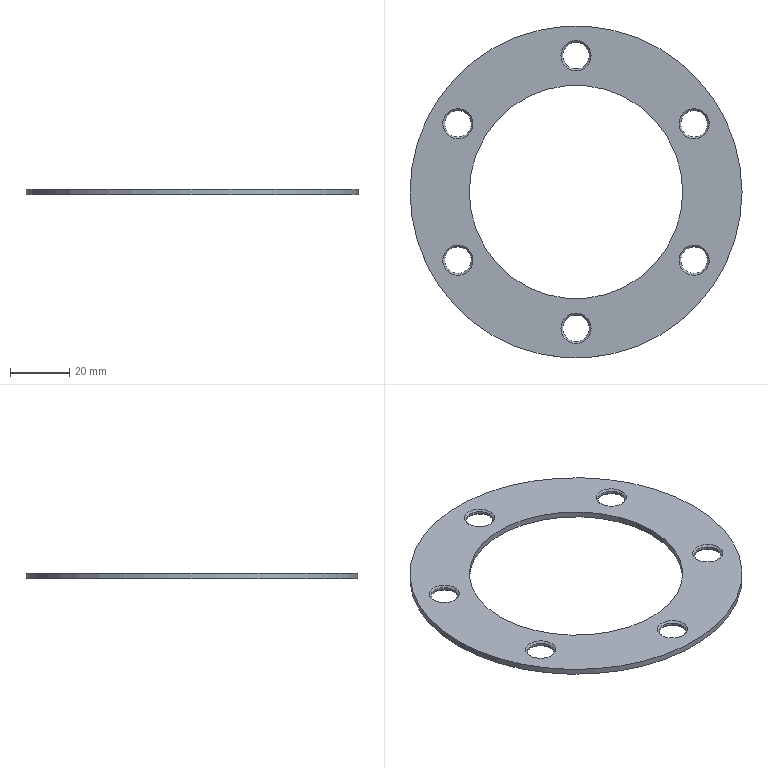Part | NX | 1 solid | 22 faces | box 112 x 112 x 2 mm | volume 10734 mm3 | cone 12 | cylinder 8 | plane 2 | commonest cylinder face diameters 9 x6 72 x1 112 x1
STEP:
#1=CARTESIAN_POINT('',(-37.287,27.417,2.));
#2=VERTEX_POINT('',#1);
#3=CARTESIAN_POINT('',(-39.837,23.,2.));
#4=DIRECTION('',(0.,0.,-1.));
#5=DIRECTION('',(0.5,0.866,0.));
#6=AXIS2_PLACEMENT_3D('',#3,#4,#5);
#7=CIRCLE('',#6,5.1);
#8=EDGE_CURVE('',#2,#2,#7,.T.);
#9=ORIENTED_EDGE('',*,*,#8,.F.);
#10=EDGE_LOOP('',(#9));
#11=FACE_BOUND('',#10,.T.);
#12=CARTESIAN_POINT('',(-37.587,26.897,1.4));
#13=VERTEX_POINT('',#12);
#14=CARTESIAN_POINT('',(-39.837,23.,1.4));
#15=DIRECTION('',(0.,0.,1.));
#16=DIRECTION('',(0.5,0.866,0.));
#17=AXIS2_PLACEMENT_3D('',#14,#15,#16);
#18=CIRCLE('',#17,4.5);
#19=EDGE_CURVE('',#13,#13,#18,.T.);
#20=ORIENTED_EDGE('',*,*,#19,.F.);
#21=EDGE_LOOP('',(#20));
#22=FACE_BOUND('',#21,.T.);
#23=CARTESIAN_POINT('',(-39.837,23.,1.4));
#24=DIRECTION('',(0.,0.,1.));
#25=DIRECTION('',(-0.5,-0.866,0.));
#26=AXIS2_PLACEMENT_3D('',#23,#24,#25);
#27=CONICAL_SURFACE('',#26,4.5,45.);
#28=ADVANCED_FACE('',(#11,#22),#27,.F.);
#29=CARTESIAN_POINT('',(-37.587,26.897,0.6));
#30=VERTEX_POINT('',#29);
#31=CARTESIAN_POINT('',(-39.837,23.,0.6));
#32=DIRECTION('',(0.,0.,-1.));
#33=DIRECTION('',(0.5,0.866,0.));
#34=AXIS2_PLACEMENT_3D('',#31,#32,#33);
#35=CIRCLE('',#34,4.5);
#36=EDGE_CURVE('',#30,#30,#35,.T.);
#37=ORIENTED_EDGE('',*,*,#36,.F.);
#38=EDGE_LOOP('',(#37));
#39=FACE_BOUND('',#38,.T.);
#40=CARTESIAN_POINT('',(-37.287,27.417,0.));
#41=VERTEX_POINT('',#40);
#42=CARTESIAN_POINT('',(-39.837,23.,0.));
#43=DIRECTION('',(0.,0.,1.));
#44=DIRECTION('',(0.5,0.866,0.));
#45=AXIS2_PLACEMENT_3D('',#42,#43,#44);
#46=CIRCLE('',#45,5.1);
#47=EDGE_CURVE('',#41,#41,#46,.T.);
#48=ORIENTED_EDGE('',*,*,#47,.F.);
#49=EDGE_LOOP('',(#48));
#50=FACE_BOUND('',#49,.T.);
#51=CARTESIAN_POINT('',(-39.837,23.,0.));
#52=DIRECTION('',(0.,0.,-1.));
#53=DIRECTION('',(0.5,0.866,0.));
#54=AXIS2_PLACEMENT_3D('',#51,#52,#53);
#55=CONICAL_SURFACE('',#54,5.1,45.);
#56=ADVANCED_FACE('',(#39,#50),#55,.F.);
#57=ORIENTED_EDGE('',*,*,#19,.T.);
#58=EDGE_LOOP('',(#57));
#59=FACE_BOUND('',#58,.T.);
#60=ORIENTED_EDGE('',*,*,#36,.T.);
#61=EDGE_LOOP('',(#60));
#62=FACE_BOUND('',#61,.T.);
#63=CARTESIAN_POINT('',(-39.837,23.,0.));
#64=DIRECTION('',(0.,0.,1.));
#65=DIRECTION('',(-0.5,-0.866,0.));
#66=AXIS2_PLACEMENT_3D('',#63,#64,#65);
#67=CYLINDRICAL_SURFACE('',#66,4.5);
#68=ADVANCED_FACE('',(#59,#62),#67,.F.);
#69=CARTESIAN_POINT('',(-42.387,-18.583,2.));
#70=VERTEX_POINT('',#69);
#71=CARTESIAN_POINT('',(-39.837,-23.,2.));
#72=DIRECTION('',(0.,0.,-1.));
#73=DIRECTION('',(-0.5,0.866,0.));
#74=AXIS2_PLACEMENT_3D('',#71,#72,#73);
#75=CIRCLE('',#74,5.1);
#76=EDGE_CURVE('',#70,#70,#75,.T.);
#77=ORIENTED_EDGE('',*,*,#76,.F.);
#78=EDGE_LOOP('',(#77));
#79=FACE_BOUND('',#78,.T.);
#80=CARTESIAN_POINT('',(-42.087,-19.103,1.4));
#81=VERTEX_POINT('',#80);
#82=CARTESIAN_POINT('',(-39.837,-23.,1.4));
#83=DIRECTION('',(0.,0.,1.));
#84=DIRECTION('',(-0.5,0.866,0.));
#85=AXIS2_PLACEMENT_3D('',#82,#83,#84);
#86=CIRCLE('',#85,4.5);
#87=EDGE_CURVE('',#81,#81,#86,.T.);
#88=ORIENTED_EDGE('',*,*,#87,.F.);
#89=EDGE_LOOP('',(#88));
#90=FACE_BOUND('',#89,.T.);
#91=CARTESIAN_POINT('',(-39.837,-23.,1.4));
#92=DIRECTION('',(0.,0.,1.));
#93=DIRECTION('',(0.5,-0.866,0.));
#94=AXIS2_PLACEMENT_3D('',#91,#92,#93);
#95=CONICAL_SURFACE('',#94,4.5,45.);
#96=ADVANCED_FACE('',(#79,#90),#95,.F.);
#97=CARTESIAN_POINT('',(-42.087,-19.103,0.6));
#98=VERTEX_POINT('',#97);
#99=CARTESIAN_POINT('',(-39.837,-23.,0.6));
#100=DIRECTION('',(0.,0.,-1.));
#101=DIRECTION('',(-0.5,0.866,0.));
#102=AXIS2_PLACEMENT_3D('',#99,#100,#101);
#103=CIRCLE('',#102,4.5);
#104=EDGE_CURVE('',#98,#98,#103,.T.);
#105=ORIENTED_EDGE('',*,*,#104,.F.);
#106=EDGE_LOOP('',(#105));
#107=FACE_BOUND('',#106,.T.);
#108=CARTESIAN_POINT('',(-42.387,-18.583,0.));
#109=VERTEX_POINT('',#108);
#110=CARTESIAN_POINT('',(-39.837,-23.,0.));
#111=DIRECTION('',(0.,0.,1.));
#112=DIRECTION('',(-0.5,0.866,0.));
#113=AXIS2_PLACEMENT_3D('',#110,#111,#112);
#114=CIRCLE('',#113,5.1);
#115=EDGE_CURVE('',#109,#109,#114,.T.);
#116=ORIENTED_EDGE('',*,*,#115,.F.);
#117=EDGE_LOOP('',(#116));
#118=FACE_BOUND('',#117,.T.);
#119=CARTESIAN_POINT('',(-39.837,-23.,0.));
#120=DIRECTION('',(0.,0.,-1.));
#121=DIRECTION('',(-0.5,0.866,0.));
#122=AXIS2_PLACEMENT_3D('',#119,#120,#121);
#123=CONICAL_SURFACE('',#122,5.1,45.);
#124=ADVANCED_FACE('',(#107,#118),#123,.F.);
#125=ORIENTED_EDGE('',*,*,#87,.T.);
#126=EDGE_LOOP('',(#125));
#127=FACE_BOUND('',#126,.T.);
#128=ORIENTED_EDGE('',*,*,#104,.T.);
#129=EDGE_LOOP('',(#128));
#130=FACE_BOUND('',#129,.T.);
#131=CARTESIAN_POINT('',(-39.837,-23.,0.));
#132=DIRECTION('',(0.,0.,1.));
#133=DIRECTION('',(0.5,-0.866,0.));
#134=AXIS2_PLACEMENT_3D('',#131,#132,#133);
#135=CYLINDRICAL_SURFACE('',#134,4.5);
#136=ADVANCED_FACE('',(#127,#130),#135,.F.);
#137=CARTESIAN_POINT('',(-5.1,-46.,2.));
#138=VERTEX_POINT('',#137);
#139=CARTESIAN_POINT('',(0.,-46.,2.));
#140=DIRECTION('',(0.,0.,-1.));
#141=DIRECTION('',(-1.,0.,0.));
#142=AXIS2_PLACEMENT_3D('',#139,#140,#141);
#143=CIRCLE('',#142,5.1);
#144=EDGE_CURVE('',#138,#138,#143,.T.);
#145=ORIENTED_EDGE('',*,*,#144,.F.);
#146=EDGE_LOOP('',(#145));
#147=FACE_BOUND('',#146,.T.);
#148=CARTESIAN_POINT('',(-4.5,-46.,1.4));
#149=VERTEX_POINT('',#148);
#150=CARTESIAN_POINT('',(0.,-46.,1.4));
#151=DIRECTION('',(0.,0.,1.));
#152=DIRECTION('',(-1.,0.,0.));
#153=AXIS2_PLACEMENT_3D('',#150,#151,#152);
#154=CIRCLE('',#153,4.5);
#155=EDGE_CURVE('',#149,#149,#154,.T.);
#156=ORIENTED_EDGE('',*,*,#155,.F.);
#157=EDGE_LOOP('',(#156));
#158=FACE_BOUND('',#157,.T.);
#159=CARTESIAN_POINT('',(0.,-46.,1.4));
#160=DIRECTION('',(0.,0.,1.));
#161=DIRECTION('',(1.,0.,0.));
#162=AXIS2_PLACEMENT_3D('',#159,#160,#161);
#163=CONICAL_SURFACE('',#162,4.5,45.);
#164=ADVANCED_FACE('',(#147,#158),#163,.F.);
#165=CARTESIAN_POINT('',(-4.5,-46.,0.6));
#166=VERTEX_POINT('',#165);
#167=CARTESIAN_POINT('',(0.,-46.,0.6));
#168=DIRECTION('',(0.,0.,-1.));
#169=DIRECTION('',(-1.,0.,0.));
#170=AXIS2_PLACEMENT_3D('',#167,#168,#169);
#171=CIRCLE('',#170,4.5);
#172=EDGE_CURVE('',#166,#166,#171,.T.);
#173=ORIENTED_EDGE('',*,*,#172,.F.);
#174=EDGE_LOOP('',(#173));
#175=FACE_BOUND('',#174,.T.);
#176=CARTESIAN_POINT('',(-5.1,-46.,0.));
#177=VERTEX_POINT('',#176);
#178=CARTESIAN_POINT('',(0.,-46.,0.));
#179=DIRECTION('',(0.,0.,1.));
#180=DIRECTION('',(-1.,0.,0.));
#181=AXIS2_PLACEMENT_3D('',#178,#179,#180);
#182=CIRCLE('',#181,5.1);
#183=EDGE_CURVE('',#177,#177,#182,.T.);
#184=ORIENTED_EDGE('',*,*,#183,.F.);
#185=EDGE_LOOP('',(#184));
#186=FACE_BOUND('',#185,.T.);
#187=CARTESIAN_POINT('',(0.,-46.,0.));
#188=DIRECTION('',(0.,0.,-1.));
#189=DIRECTION('',(-1.,0.,0.));
#190=AXIS2_PLACEMENT_3D('',#187,#188,#189);
#191=CONICAL_SURFACE('',#190,5.1,45.);
#192=ADVANCED_FACE('',(#175,#186),#191,.F.);
#193=ORIENTED_EDGE('',*,*,#155,.T.);
#194=EDGE_LOOP('',(#193));
#195=FACE_BOUND('',#194,.T.);
#196=ORIENTED_EDGE('',*,*,#172,.T.);
#197=EDGE_LOOP('',(#196));
#198=FACE_BOUND('',#197,.T.);
#199=CARTESIAN_POINT('',(0.,-46.,0.));
#200=DIRECTION('',(0.,0.,1.));
#201=DIRECTION('',(1.,0.,0.));
#202=AXIS2_PLACEMENT_3D('',#199,#200,#201);
#203=CYLINDRICAL_SURFACE('',#202,4.5);
#204=ADVANCED_FACE('',(#195,#198),#203,.F.);
#205=CARTESIAN_POINT('',(37.287,-27.417,2.));
#206=VERTEX_POINT('',#205);
#207=CARTESIAN_POINT('',(39.837,-23.,2.));
#208=DIRECTION('',(0.,0.,-1.));
#209=DIRECTION('',(-0.5,-0.866,0.));
#210=AXIS2_PLACEMENT_3D('',#207,#208,#209);
#211=CIRCLE('',#210,5.1);
#212=EDGE_CURVE('',#206,#206,#211,.T.);
#213=ORIENTED_EDGE('',*,*,#212,.F.);
#214=EDGE_LOOP('',(#213));
#215=FACE_BOUND('',#214,.T.);
#216=CARTESIAN_POINT('',(37.587,-26.897,1.4));
#217=VERTEX_POINT('',#216);
#218=CARTESIAN_POINT('',(39.837,-23.,1.4));
#219=DIRECTION('',(0.,0.,1.));
#220=DIRECTION('',(-0.5,-0.866,0.));
#221=AXIS2_PLACEMENT_3D('',#218,#219,#220);
#222=CIRCLE('',#221,4.5);
#223=EDGE_CURVE('',#217,#217,#222,.T.);
#224=ORIENTED_EDGE('',*,*,#223,.F.);
#225=EDGE_LOOP('',(#224));
#226=FACE_BOUND('',#225,.T.);
#227=CARTESIAN_POINT('',(39.837,-23.,1.4));
#228=DIRECTION('',(0.,0.,1.));
#229=DIRECTION('',(0.5,0.866,0.));
#230=AXIS2_PLACEMENT_3D('',#227,#228,#229);
#231=CONICAL_SURFACE('',#230,4.5,45.);
#232=ADVANCED_FACE('',(#215,#226),#231,.F.);
#233=CARTESIAN_POINT('',(37.587,-26.897,0.6));
#234=VERTEX_POINT('',#233);
#235=CARTESIAN_POINT('',(39.837,-23.,0.6));
#236=DIRECTION('',(0.,0.,-1.));
#237=DIRECTION('',(-0.5,-0.866,0.));
#238=AXIS2_PLACEMENT_3D('',#235,#236,#237);
#239=CIRCLE('',#238,4.5);
#240=EDGE_CURVE('',#234,#234,#239,.T.);
#241=ORIENTED_EDGE('',*,*,#240,.F.);
#242=EDGE_LOOP('',(#241));
#243=FACE_BOUND('',#242,.T.);
#244=CARTESIAN_POINT('',(37.287,-27.417,0.));
#245=VERTEX_POINT('',#244);
#246=CARTESIAN_POINT('',(39.837,-23.,0.));
#247=DIRECTION('',(0.,0.,1.));
#248=DIRECTION('',(-0.5,-0.866,0.));
#249=AXIS2_PLACEMENT_3D('',#246,#247,#248);
#250=CIRCLE('',#249,5.1);
#251=EDGE_CURVE('',#245,#245,#250,.T.);
#252=ORIENTED_EDGE('',*,*,#251,.F.);
#253=EDGE_LOOP('',(#252));
#254=FACE_BOUND('',#253,.T.);
#255=CARTESIAN_POINT('',(39.837,-23.,0.));
#256=DIRECTION('',(0.,0.,-1.));
#257=DIRECTION('',(-0.5,-0.866,0.));
#258=AXIS2_PLACEMENT_3D('',#255,#256,#257);
#259=CONICAL_SURFACE('',#258,5.1,45.);
#260=ADVANCED_FACE('',(#243,#254),#259,.F.);
#261=ORIENTED_EDGE('',*,*,#223,.T.);
#262=EDGE_LOOP('',(#261));
#263=FACE_BOUND('',#262,.T.);
#264=ORIENTED_EDGE('',*,*,#240,.T.);
#265=EDGE_LOOP('',(#264));
#266=FACE_BOUND('',#265,.T.);
#267=CARTESIAN_POINT('',(39.837,-23.,0.));
#268=DIRECTION('',(0.,0.,1.));
#269=DIRECTION('',(0.5,0.866,0.));
#270=AXIS2_PLACEMENT_3D('',#267,#268,#269);
#271=CYLINDRICAL_SURFACE('',#270,4.5);
#272=ADVANCED_FACE('',(#263,#266),#271,.F.);
#273=CARTESIAN_POINT('',(42.387,18.583,2.));
#274=VERTEX_POINT('',#273);
#275=CARTESIAN_POINT('',(39.837,23.,2.));
#276=DIRECTION('',(0.,0.,-1.));
#277=DIRECTION('',(0.5,-0.866,0.));
#278=AXIS2_PLACEMENT_3D('',#275,#276,#277);
#279=CIRCLE('',#278,5.1);
#280=EDGE_CURVE('',#274,#274,#279,.T.);
#281=ORIENTED_EDGE('',*,*,#280,.F.);
#282=EDGE_LOOP('',(#281));
#283=FACE_BOUND('',#282,.T.);
#284=CARTESIAN_POINT('',(42.087,19.103,1.4));
#285=VERTEX_POINT('',#284);
#286=CARTESIAN_POINT('',(39.837,23.,1.4));
#287=DIRECTION('',(0.,0.,1.));
#288=DIRECTION('',(0.5,-0.866,0.));
#289=AXIS2_PLACEMENT_3D('',#286,#287,#288);
#290=CIRCLE('',#289,4.5);
#291=EDGE_CURVE('',#285,#285,#290,.T.);
#292=ORIENTED_EDGE('',*,*,#291,.F.);
#293=EDGE_LOOP('',(#292));
#294=FACE_BOUND('',#293,.T.);
#295=CARTESIAN_POINT('',(39.837,23.,1.4));
#296=DIRECTION('',(0.,0.,1.));
#297=DIRECTION('',(-0.5,0.866,0.));
#298=AXIS2_PLACEMENT_3D('',#295,#296,#297);
#299=CONICAL_SURFACE('',#298,4.5,45.);
#300=ADVANCED_FACE('',(#283,#294),#299,.F.);
#301=CARTESIAN_POINT('',(42.087,19.103,0.6));
#302=VERTEX_POINT('',#301);
#303=CARTESIAN_POINT('',(39.837,23.,0.6));
#304=DIRECTION('',(0.,0.,-1.));
#305=DIRECTION('',(0.5,-0.866,0.));
#306=AXIS2_PLACEMENT_3D('',#303,#304,#305);
#307=CIRCLE('',#306,4.5);
#308=EDGE_CURVE('',#302,#302,#307,.T.);
#309=ORIENTED_EDGE('',*,*,#308,.F.);
#310=EDGE_LOOP('',(#309));
#311=FACE_BOUND('',#310,.T.);
#312=CARTESIAN_POINT('',(42.387,18.583,0.));
#313=VERTEX_POINT('',#312);
#314=CARTESIAN_POINT('',(39.837,23.,0.));
#315=DIRECTION('',(0.,0.,1.));
#316=DIRECTION('',(0.5,-0.866,0.));
#317=AXIS2_PLACEMENT_3D('',#314,#315,#316);
#318=CIRCLE('',#317,5.1);
#319=EDGE_CURVE('',#313,#313,#318,.T.);
#320=ORIENTED_EDGE('',*,*,#319,.F.);
#321=EDGE_LOOP('',(#320));
#322=FACE_BOUND('',#321,.T.);
#323=CARTESIAN_POINT('',(39.837,23.,0.));
#324=DIRECTION('',(0.,0.,-1.));
#325=DIRECTION('',(0.5,-0.866,0.));
#326=AXIS2_PLACEMENT_3D('',#323,#324,#325);
#327=CONICAL_SURFACE('',#326,5.1,45.);
#328=ADVANCED_FACE('',(#311,#322),#327,.F.);
#329=ORIENTED_EDGE('',*,*,#291,.T.);
#330=EDGE_LOOP('',(#329));
#331=FACE_BOUND('',#330,.T.);
#332=ORIENTED_EDGE('',*,*,#308,.T.);
#333=EDGE_LOOP('',(#332));
#334=FACE_BOUND('',#333,.T.);
#335=CARTESIAN_POINT('',(39.837,23.,0.));
#336=DIRECTION('',(0.,0.,1.));
#337=DIRECTION('',(-0.5,0.866,0.));
#338=AXIS2_PLACEMENT_3D('',#335,#336,#337);
#339=CYLINDRICAL_SURFACE('',#338,4.5);
#340=ADVANCED_FACE('',(#331,#334),#339,.F.);
#341=CARTESIAN_POINT('',(56.,0.,2.));
#342=VERTEX_POINT('',#341);
#343=CARTESIAN_POINT('',(0.,0.,2.));
#344=DIRECTION('',(0.,0.,1.));
#345=DIRECTION('',(1.,0.,0.));
#346=AXIS2_PLACEMENT_3D('',#343,#344,#345);
#347=CIRCLE('',#346,56.);
#348=EDGE_CURVE('',#342,#342,#347,.T.);
#349=ORIENTED_EDGE('',*,*,#348,.F.);
#350=EDGE_LOOP('',(#349));
#351=FACE_BOUND('',#350,.T.);
#352=CARTESIAN_POINT('',(56.,0.,0.));
#353=VERTEX_POINT('',#352);
#354=CARTESIAN_POINT('',(0.,0.,0.));
#355=DIRECTION('',(0.,0.,1.));
#356=DIRECTION('',(1.,0.,0.));
#357=AXIS2_PLACEMENT_3D('',#354,#355,#356);
#358=CIRCLE('',#357,56.);
#359=EDGE_CURVE('',#353,#353,#358,.T.);
#360=ORIENTED_EDGE('',*,*,#359,.T.);
#361=EDGE_LOOP('',(#360));
#362=FACE_BOUND('',#361,.T.);
#363=CARTESIAN_POINT('',(0.,0.,2.));
#364=DIRECTION('',(0.,0.,-1.));
#365=DIRECTION('',(1.,0.,0.));
#366=AXIS2_PLACEMENT_3D('',#363,#364,#365);
#367=CYLINDRICAL_SURFACE('',#366,56.);
#368=ADVANCED_FACE('',(#351,#362),#367,.T.);
#369=CARTESIAN_POINT('',(36.,0.,2.));
#370=VERTEX_POINT('',#369);
#371=CARTESIAN_POINT('',(0.,0.,2.));
#372=DIRECTION('',(0.,0.,1.));
#373=DIRECTION('',(1.,0.,0.));
#374=AXIS2_PLACEMENT_3D('',#371,#372,#373);
#375=CIRCLE('',#374,36.);
#376=EDGE_CURVE('',#370,#370,#375,.T.);
#377=ORIENTED_EDGE('',*,*,#376,.T.);
#378=EDGE_LOOP('',(#377));
#379=FACE_BOUND('',#378,.T.);
#380=CARTESIAN_POINT('',(36.,0.,0.));
#381=VERTEX_POINT('',#380);
#382=CARTESIAN_POINT('',(0.,0.,0.));
#383=DIRECTION('',(0.,0.,1.));
#384=DIRECTION('',(1.,0.,0.));
#385=AXIS2_PLACEMENT_3D('',#382,#383,#384);
#386=CIRCLE('',#385,36.);
#387=EDGE_CURVE('',#381,#381,#386,.T.);
#388=ORIENTED_EDGE('',*,*,#387,.F.);
#389=EDGE_LOOP('',(#388));
#390=FACE_BOUND('',#389,.T.);
#391=CARTESIAN_POINT('',(0.,0.,2.));
#392=DIRECTION('',(0.,0.,-1.));
#393=DIRECTION('',(1.,0.,0.));
#394=AXIS2_PLACEMENT_3D('',#391,#392,#393);
#395=CYLINDRICAL_SURFACE('',#394,36.);
#396=ADVANCED_FACE('',(#379,#390),#395,.F.);
#397=ORIENTED_EDGE('',*,*,#8,.T.);
#398=EDGE_LOOP('',(#397));
#399=FACE_BOUND('',#398,.T.);
#400=ORIENTED_EDGE('',*,*,#76,.T.);
#401=EDGE_LOOP('',(#400));
#402=FACE_BOUND('',#401,.T.);
#403=ORIENTED_EDGE('',*,*,#144,.T.);
#404=EDGE_LOOP('',(#403));
#405=FACE_BOUND('',#404,.T.);
#406=ORIENTED_EDGE('',*,*,#212,.T.);
#407=EDGE_LOOP('',(#406));
#408=FACE_BOUND('',#407,.T.);
#409=ORIENTED_EDGE('',*,*,#280,.T.);
#410=EDGE_LOOP('',(#409));
#411=FACE_BOUND('',#410,.T.);
#412=CARTESIAN_POINT('',(5.1,46.,2.));
#413=VERTEX_POINT('',#412);
#414=CARTESIAN_POINT('',(0.,46.,2.));
#415=DIRECTION('',(0.,0.,-1.));
#416=DIRECTION('',(1.,0.,0.));
#417=AXIS2_PLACEMENT_3D('',#414,#415,#416);
#418=CIRCLE('',#417,5.1);
#419=EDGE_CURVE('',#413,#413,#418,.T.);
#420=ORIENTED_EDGE('',*,*,#419,.T.);
#421=EDGE_LOOP('',(#420));
#422=FACE_BOUND('',#421,.T.);
#423=ORIENTED_EDGE('',*,*,#348,.T.);
#424=EDGE_LOOP('',(#423));
#425=FACE_BOUND('',#424,.T.);
#426=ORIENTED_EDGE('',*,*,#376,.F.);
#427=EDGE_LOOP('',(#426));
#428=FACE_BOUND('',#427,.T.);
#429=CARTESIAN_POINT('',(0.,0.,2.));
#430=DIRECTION('',(0.,0.,1.));
#431=DIRECTION('',(-1.,0.,0.));
#432=AXIS2_PLACEMENT_3D('',#429,#430,#431);
#433=PLANE('',#432);
#434=ADVANCED_FACE('',(#399,#402,#405,#408,#411,#422,#425,#428),#433,.T.);
#435=ORIENTED_EDGE('',*,*,#47,.T.);
#436=EDGE_LOOP('',(#435));
#437=FACE_BOUND('',#436,.T.);
#438=ORIENTED_EDGE('',*,*,#115,.T.);
#439=EDGE_LOOP('',(#438));
#440=FACE_BOUND('',#439,.T.);
#441=ORIENTED_EDGE('',*,*,#183,.T.);
#442=EDGE_LOOP('',(#441));
#443=FACE_BOUND('',#442,.T.);
#444=ORIENTED_EDGE('',*,*,#251,.T.);
#445=EDGE_LOOP('',(#444));
#446=FACE_BOUND('',#445,.T.);
#447=ORIENTED_EDGE('',*,*,#319,.T.);
#448=EDGE_LOOP('',(#447));
#449=FACE_BOUND('',#448,.T.);
#450=CARTESIAN_POINT('',(5.1,46.,0.));
#451=VERTEX_POINT('',#450);
#452=CARTESIAN_POINT('',(0.,46.,0.));
#453=DIRECTION('',(0.,0.,1.));
#454=DIRECTION('',(1.,0.,0.));
#455=AXIS2_PLACEMENT_3D('',#452,#453,#454);
#456=CIRCLE('',#455,5.1);
#457=EDGE_CURVE('',#451,#451,#456,.T.);
#458=ORIENTED_EDGE('',*,*,#457,.T.);
#459=EDGE_LOOP('',(#458));
#460=FACE_BOUND('',#459,.T.);
#461=ORIENTED_EDGE('',*,*,#359,.F.);
#462=EDGE_LOOP('',(#461));
#463=FACE_BOUND('',#462,.T.);
#464=ORIENTED_EDGE('',*,*,#387,.T.);
#465=EDGE_LOOP('',(#464));
#466=FACE_BOUND('',#465,.T.);
#467=CARTESIAN_POINT('',(0.,0.,0.));
#468=DIRECTION('',(0.,0.,1.));
#469=DIRECTION('',(-1.,0.,0.));
#470=AXIS2_PLACEMENT_3D('',#467,#468,#469);
#471=PLANE('',#470);
#472=ADVANCED_FACE('',(#437,#440,#443,#446,#449,#460,#463,#466),#471,.F.);
#473=CARTESIAN_POINT('',(4.5,46.,1.4));
#474=VERTEX_POINT('',#473);
#475=CARTESIAN_POINT('',(0.,46.,1.4));
#476=DIRECTION('',(0.,0.,1.));
#477=DIRECTION('',(1.,0.,0.));
#478=AXIS2_PLACEMENT_3D('',#475,#476,#477);
#479=CIRCLE('',#478,4.5);
#480=EDGE_CURVE('',#474,#474,#479,.T.);
#481=ORIENTED_EDGE('',*,*,#480,.T.);
#482=EDGE_LOOP('',(#481));
#483=FACE_BOUND('',#482,.T.);
#484=CARTESIAN_POINT('',(4.5,46.,0.6));
#485=VERTEX_POINT('',#484);
#486=CARTESIAN_POINT('',(0.,46.,0.6));
#487=DIRECTION('',(0.,0.,-1.));
#488=DIRECTION('',(1.,0.,0.));
#489=AXIS2_PLACEMENT_3D('',#486,#487,#488);
#490=CIRCLE('',#489,4.5);
#491=EDGE_CURVE('',#485,#485,#490,.T.);
#492=ORIENTED_EDGE('',*,*,#491,.T.);
#493=EDGE_LOOP('',(#492));
#494=FACE_BOUND('',#493,.T.);
#495=CARTESIAN_POINT('',(0.,46.,0.));
#496=DIRECTION('',(0.,0.,1.));
#497=DIRECTION('',(-1.,0.,0.));
#498=AXIS2_PLACEMENT_3D('',#495,#496,#497);
#499=CYLINDRICAL_SURFACE('',#498,4.5);
#500=ADVANCED_FACE('',(#483,#494),#499,.F.);
#501=ORIENTED_EDGE('',*,*,#491,.F.);
#502=EDGE_LOOP('',(#501));
#503=FACE_BOUND('',#502,.T.);
#504=ORIENTED_EDGE('',*,*,#457,.F.);
#505=EDGE_LOOP('',(#504));
#506=FACE_BOUND('',#505,.T.);
#507=CARTESIAN_POINT('',(0.,46.,0.));
#508=DIRECTION('',(0.,0.,-1.));
#509=DIRECTION('',(1.,0.,0.));
#510=AXIS2_PLACEMENT_3D('',#507,#508,#509);
#511=CONICAL_SURFACE('',#510,5.1,45.);
#512=ADVANCED_FACE('',(#503,#506),#511,.F.);
#513=ORIENTED_EDGE('',*,*,#419,.F.);
#514=EDGE_LOOP('',(#513));
#515=FACE_BOUND('',#514,.T.);
#516=ORIENTED_EDGE('',*,*,#480,.F.);
#517=EDGE_LOOP('',(#516));
#518=FACE_BOUND('',#517,.T.);
#519=CARTESIAN_POINT('',(0.,46.,1.4));
#520=DIRECTION('',(0.,0.,1.));
#521=DIRECTION('',(-1.,0.,0.));
#522=AXIS2_PLACEMENT_3D('',#519,#520,#521);
#523=CONICAL_SURFACE('',#522,4.5,45.);
#524=ADVANCED_FACE('',(#515,#518),#523,.F.);
#525=CLOSED_SHELL('',(#28,#56,#68,#96,#124,#136,#164,#192,#204,#232,#260,#272,#300,#328,#340,#368,#396,#434,#472,#500,#512,#524));
#526=MANIFOLD_SOLID_BREP('',#525);
#527=(LENGTH_UNIT()NAMED_UNIT(*)SI_UNIT(.MILLI.,.METRE.));
#528=UNCERTAINTY_MEASURE_WITH_UNIT(LENGTH_MEASURE(0.00002),#527,'','');
#529=(NAMED_UNIT(*)PLANE_ANGLE_UNIT()SI_UNIT($,.RADIAN.));
#530=PLANE_ANGLE_MEASURE_WITH_UNIT(PLANE_ANGLE_MEASURE(0.01745),#529);
#531=DIMENSIONAL_EXPONENTS(0.,0.,0.,0.,0.,0.,0.);
#532=(CONVERSION_BASED_UNIT('DEGREE',#530)NAMED_UNIT(#531)PLANE_ANGLE_UNIT());
#533=(NAMED_UNIT(*)SI_UNIT($,.STERADIAN.)SOLID_ANGLE_UNIT());
#534=(GEOMETRIC_REPRESENTATION_CONTEXT(3)GLOBAL_UNCERTAINTY_ASSIGNED_CONTEXT((#528))GLOBAL_UNIT_ASSIGNED_CONTEXT((#527,#532,#533))REPRESENTATION_CONTEXT('',''));
#535=ADVANCED_BREP_SHAPE_REPRESENTATION('',(#526),#534);